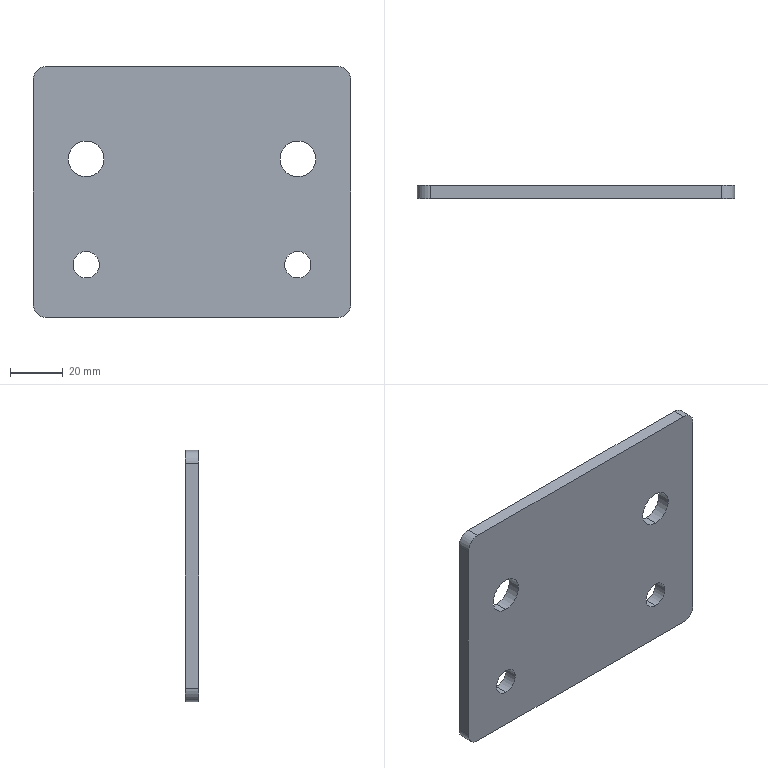Part | 1 solid | 18 faces | box 120 x 5 x 95 mm | volume 54676 mm3 | cylinder 12 | plane 6 | commonest cylinder face diameters 10 x8 13.5 x4
STEP:
#1=CARTESIAN_POINT('',(-40.,0.,-65.));
#2=VERTEX_POINT('',#1);
#3=CARTESIAN_POINT('',(-40.,0.,-75.));
#4=VERTEX_POINT('',#3);
#5=CARTESIAN_POINT('',(-40.,0.,-70.));
#6=DIRECTION('',(0.,-1.,0.));
#7=DIRECTION('',(0.,0.,-1.));
#8=AXIS2_PLACEMENT_3D('',#5,#6,#7);
#9=CIRCLE('',#8,5.);
#10=EDGE_CURVE('',#2,#4,#9,.T.);
#11=ORIENTED_EDGE('',*,*,#10,.F.);
#12=CARTESIAN_POINT('',(-40.,-5.,-65.));
#13=VERTEX_POINT('',#12);
#14=CARTESIAN_POINT('',(-40.,0.,-65.));
#15=DIRECTION('',(0.,-1.,0.));
#16=VECTOR('',#15,1000.);
#17=LINE('',#14,#16);
#18=EDGE_CURVE('',#2,#13,#17,.T.);
#19=ORIENTED_EDGE('',*,*,#18,.T.);
#20=CARTESIAN_POINT('',(-40.,-5.,-75.));
#21=VERTEX_POINT('',#20);
#22=CARTESIAN_POINT('',(-40.,-5.,-70.));
#23=DIRECTION('',(0.,-1.,0.));
#24=DIRECTION('',(0.,0.,-1.));
#25=AXIS2_PLACEMENT_3D('',#22,#23,#24);
#26=CIRCLE('',#25,5.);
#27=EDGE_CURVE('',#13,#21,#26,.T.);
#28=ORIENTED_EDGE('',*,*,#27,.T.);
#29=CARTESIAN_POINT('',(-40.,0.,-75.));
#30=DIRECTION('',(0.,-1.,0.));
#31=VECTOR('',#30,1000.);
#32=LINE('',#29,#31);
#33=EDGE_CURVE('',#4,#21,#32,.T.);
#34=ORIENTED_EDGE('',*,*,#33,.F.);
#35=EDGE_LOOP('',(#11,#19,#28,#34));
#36=FACE_OUTER_BOUND('',#35,.T.);
#37=CARTESIAN_POINT('',(-40.,0.,-70.));
#38=DIRECTION('',(0.,-1.,0.));
#39=DIRECTION('',(0.,0.,-1.));
#40=AXIS2_PLACEMENT_3D('',#37,#38,#39);
#41=CYLINDRICAL_SURFACE('',#40,5.);
#42=ADVANCED_FACE('',(#36),#41,.F.);
#43=CARTESIAN_POINT('',(40.,0.,-65.));
#44=VERTEX_POINT('',#43);
#45=CARTESIAN_POINT('',(40.,0.,-75.));
#46=VERTEX_POINT('',#45);
#47=CARTESIAN_POINT('',(40.,0.,-70.));
#48=DIRECTION('',(0.,-1.,0.));
#49=DIRECTION('',(0.,0.,-1.));
#50=AXIS2_PLACEMENT_3D('',#47,#48,#49);
#51=CIRCLE('',#50,5.);
#52=EDGE_CURVE('',#44,#46,#51,.T.);
#53=ORIENTED_EDGE('',*,*,#52,.F.);
#54=CARTESIAN_POINT('',(40.,-5.,-65.));
#55=VERTEX_POINT('',#54);
#56=CARTESIAN_POINT('',(40.,0.,-65.));
#57=DIRECTION('',(0.,-1.,0.));
#58=VECTOR('',#57,1000.);
#59=LINE('',#56,#58);
#60=EDGE_CURVE('',#44,#55,#59,.T.);
#61=ORIENTED_EDGE('',*,*,#60,.T.);
#62=CARTESIAN_POINT('',(40.,-5.,-75.));
#63=VERTEX_POINT('',#62);
#64=CARTESIAN_POINT('',(40.,-5.,-70.));
#65=DIRECTION('',(0.,-1.,0.));
#66=DIRECTION('',(0.,0.,-1.));
#67=AXIS2_PLACEMENT_3D('',#64,#65,#66);
#68=CIRCLE('',#67,5.);
#69=EDGE_CURVE('',#55,#63,#68,.T.);
#70=ORIENTED_EDGE('',*,*,#69,.T.);
#71=CARTESIAN_POINT('',(40.,0.,-75.));
#72=DIRECTION('',(0.,-1.,0.));
#73=VECTOR('',#72,1000.);
#74=LINE('',#71,#73);
#75=EDGE_CURVE('',#46,#63,#74,.T.);
#76=ORIENTED_EDGE('',*,*,#75,.F.);
#77=EDGE_LOOP('',(#53,#61,#70,#76));
#78=FACE_OUTER_BOUND('',#77,.T.);
#79=CARTESIAN_POINT('',(40.,0.,-70.));
#80=DIRECTION('',(0.,-1.,0.));
#81=DIRECTION('',(0.,0.,-1.));
#82=AXIS2_PLACEMENT_3D('',#79,#80,#81);
#83=CYLINDRICAL_SURFACE('',#82,5.);
#84=ADVANCED_FACE('',(#78),#83,.F.);
#85=CARTESIAN_POINT('',(40.,0.,-23.25));
#86=VERTEX_POINT('',#85);
#87=CARTESIAN_POINT('',(40.,0.,-36.75));
#88=VERTEX_POINT('',#87);
#89=CARTESIAN_POINT('',(40.,0.,-30.));
#90=DIRECTION('',(0.,-1.,0.));
#91=DIRECTION('',(0.,0.,-1.));
#92=AXIS2_PLACEMENT_3D('',#89,#90,#91);
#93=CIRCLE('',#92,6.75);
#94=EDGE_CURVE('',#86,#88,#93,.T.);
#95=ORIENTED_EDGE('',*,*,#94,.F.);
#96=CARTESIAN_POINT('',(40.,-5.,-23.25));
#97=VERTEX_POINT('',#96);
#98=CARTESIAN_POINT('',(40.,-5.,-23.25));
#99=DIRECTION('',(0.,-1.,0.));
#100=VECTOR('',#99,1000.);
#101=LINE('',#98,#100);
#102=EDGE_CURVE('',#86,#97,#101,.T.);
#103=ORIENTED_EDGE('',*,*,#102,.T.);
#104=CARTESIAN_POINT('',(40.,-5.,-36.75));
#105=VERTEX_POINT('',#104);
#106=CARTESIAN_POINT('',(40.,-5.,-30.));
#107=DIRECTION('',(0.,-1.,0.));
#108=DIRECTION('',(0.,0.,-1.));
#109=AXIS2_PLACEMENT_3D('',#106,#107,#108);
#110=CIRCLE('',#109,6.75);
#111=EDGE_CURVE('',#97,#105,#110,.T.);
#112=ORIENTED_EDGE('',*,*,#111,.T.);
#113=CARTESIAN_POINT('',(40.,-5.,-36.75));
#114=DIRECTION('',(0.,-1.,0.));
#115=VECTOR('',#114,1000.);
#116=LINE('',#113,#115);
#117=EDGE_CURVE('',#88,#105,#116,.T.);
#118=ORIENTED_EDGE('',*,*,#117,.F.);
#119=EDGE_LOOP('',(#95,#103,#112,#118));
#120=FACE_OUTER_BOUND('',#119,.T.);
#121=CARTESIAN_POINT('',(40.,-5.,-30.));
#122=DIRECTION('',(0.,-1.,0.));
#123=DIRECTION('',(0.,0.,-1.));
#124=AXIS2_PLACEMENT_3D('',#121,#122,#123);
#125=CYLINDRICAL_SURFACE('',#124,6.75);
#126=ADVANCED_FACE('',(#120),#125,.F.);
#127=CARTESIAN_POINT('',(-40.,0.,-23.25));
#128=VERTEX_POINT('',#127);
#129=CARTESIAN_POINT('',(-40.,0.,-36.75));
#130=VERTEX_POINT('',#129);
#131=CARTESIAN_POINT('',(-40.,0.,-30.));
#132=DIRECTION('',(0.,-1.,0.));
#133=DIRECTION('',(0.,0.,-1.));
#134=AXIS2_PLACEMENT_3D('',#131,#132,#133);
#135=CIRCLE('',#134,6.75);
#136=EDGE_CURVE('',#128,#130,#135,.T.);
#137=ORIENTED_EDGE('',*,*,#136,.F.);
#138=CARTESIAN_POINT('',(-40.,-5.,-23.25));
#139=VERTEX_POINT('',#138);
#140=CARTESIAN_POINT('',(-40.,-5.,-23.25));
#141=DIRECTION('',(0.,-1.,0.));
#142=VECTOR('',#141,1000.);
#143=LINE('',#140,#142);
#144=EDGE_CURVE('',#128,#139,#143,.T.);
#145=ORIENTED_EDGE('',*,*,#144,.T.);
#146=CARTESIAN_POINT('',(-40.,-5.,-36.75));
#147=VERTEX_POINT('',#146);
#148=CARTESIAN_POINT('',(-40.,-5.,-30.));
#149=DIRECTION('',(0.,-1.,0.));
#150=DIRECTION('',(0.,0.,-1.));
#151=AXIS2_PLACEMENT_3D('',#148,#149,#150);
#152=CIRCLE('',#151,6.75);
#153=EDGE_CURVE('',#139,#147,#152,.T.);
#154=ORIENTED_EDGE('',*,*,#153,.T.);
#155=CARTESIAN_POINT('',(-40.,-5.,-36.75));
#156=DIRECTION('',(0.,-1.,0.));
#157=VECTOR('',#156,1000.);
#158=LINE('',#155,#157);
#159=EDGE_CURVE('',#130,#147,#158,.T.);
#160=ORIENTED_EDGE('',*,*,#159,.F.);
#161=EDGE_LOOP('',(#137,#145,#154,#160));
#162=FACE_OUTER_BOUND('',#161,.T.);
#163=CARTESIAN_POINT('',(-40.,-5.,-30.));
#164=DIRECTION('',(0.,-1.,0.));
#165=DIRECTION('',(0.,0.,-1.));
#166=AXIS2_PLACEMENT_3D('',#163,#164,#165);
#167=CYLINDRICAL_SURFACE('',#166,6.75);
#168=ADVANCED_FACE('',(#162),#167,.F.);
#169=CARTESIAN_POINT('',(60.,0.,0.));
#170=VERTEX_POINT('',#169);
#171=CARTESIAN_POINT('',(60.,0.,-85.));
#172=VERTEX_POINT('',#171);
#173=CARTESIAN_POINT('',(60.,0.,50.));
#174=DIRECTION('',(0.,0.,-1.));
#175=VECTOR('',#174,1000.);
#176=LINE('',#173,#175);
#177=EDGE_CURVE('',#170,#172,#176,.T.);
#178=ORIENTED_EDGE('',*,*,#177,.F.);
#179=CARTESIAN_POINT('',(60.,-5.,0.));
#180=VERTEX_POINT('',#179);
#181=CARTESIAN_POINT('',(60.,-5.,0.));
#182=DIRECTION('',(0.,-1.,0.));
#183=VECTOR('',#182,1000.);
#184=LINE('',#181,#183);
#185=EDGE_CURVE('',#170,#180,#184,.T.);
#186=ORIENTED_EDGE('',*,*,#185,.T.);
#187=CARTESIAN_POINT('',(60.,-5.,-85.));
#188=VERTEX_POINT('',#187);
#189=CARTESIAN_POINT('',(60.,-5.,50.));
#190=DIRECTION('',(0.,0.,-1.));
#191=VECTOR('',#190,1000.);
#192=LINE('',#189,#191);
#193=EDGE_CURVE('',#180,#188,#192,.T.);
#194=ORIENTED_EDGE('',*,*,#193,.T.);
#195=CARTESIAN_POINT('',(60.,-5.,-85.));
#196=DIRECTION('',(0.,1.,0.));
#197=VECTOR('',#196,1000.);
#198=LINE('',#195,#197);
#199=EDGE_CURVE('',#188,#172,#198,.T.);
#200=ORIENTED_EDGE('',*,*,#199,.T.);
#201=EDGE_LOOP('',(#178,#186,#194,#200));
#202=FACE_OUTER_BOUND('',#201,.T.);
#203=CARTESIAN_POINT('',(60.,-5.,50.));
#204=DIRECTION('',(1.,0.,0.));
#205=DIRECTION('',(0.,0.,-1.));
#206=AXIS2_PLACEMENT_3D('',#203,#204,#205);
#207=PLANE('',#206);
#208=ADVANCED_FACE('',(#202),#207,.T.);
#209=CARTESIAN_POINT('',(-60.,0.,-85.));
#210=VERTEX_POINT('',#209);
#211=CARTESIAN_POINT('',(-60.,0.,0.));
#212=VERTEX_POINT('',#211);
#213=CARTESIAN_POINT('',(-60.,0.,50.));
#214=DIRECTION('',(0.,0.,1.));
#215=VECTOR('',#214,1000.);
#216=LINE('',#213,#215);
#217=EDGE_CURVE('',#210,#212,#216,.T.);
#218=ORIENTED_EDGE('',*,*,#217,.F.);
#219=CARTESIAN_POINT('',(-60.,-5.,-85.));
#220=VERTEX_POINT('',#219);
#221=CARTESIAN_POINT('',(-60.,-5.,-85.));
#222=DIRECTION('',(0.,-1.,0.));
#223=VECTOR('',#222,1000.);
#224=LINE('',#221,#223);
#225=EDGE_CURVE('',#210,#220,#224,.T.);
#226=ORIENTED_EDGE('',*,*,#225,.T.);
#227=CARTESIAN_POINT('',(-60.,-5.,0.));
#228=VERTEX_POINT('',#227);
#229=CARTESIAN_POINT('',(-60.,-5.,50.));
#230=DIRECTION('',(0.,0.,1.));
#231=VECTOR('',#230,1000.);
#232=LINE('',#229,#231);
#233=EDGE_CURVE('',#220,#228,#232,.T.);
#234=ORIENTED_EDGE('',*,*,#233,.T.);
#235=CARTESIAN_POINT('',(-60.,0.,0.));
#236=DIRECTION('',(0.,1.,0.));
#237=VECTOR('',#236,1000.);
#238=LINE('',#235,#237);
#239=EDGE_CURVE('',#228,#212,#238,.T.);
#240=ORIENTED_EDGE('',*,*,#239,.T.);
#241=EDGE_LOOP('',(#218,#226,#234,#240));
#242=FACE_OUTER_BOUND('',#241,.T.);
#243=CARTESIAN_POINT('',(-60.,-5.,50.));
#244=DIRECTION('',(-1.,0.,0.));
#245=DIRECTION('',(0.,0.,1.));
#246=AXIS2_PLACEMENT_3D('',#243,#244,#245);
#247=PLANE('',#246);
#248=ADVANCED_FACE('',(#242),#247,.T.);
#249=CARTESIAN_POINT('',(55.,-5.,-90.));
#250=VERTEX_POINT('',#249);
#251=CARTESIAN_POINT('',(-55.,-5.,-90.));
#252=VERTEX_POINT('',#251);
#253=CARTESIAN_POINT('',(-60.,-5.,-90.));
#254=DIRECTION('',(-1.,0.,0.));
#255=VECTOR('',#254,1000.);
#256=LINE('',#253,#255);
#257=EDGE_CURVE('',#250,#252,#256,.T.);
#258=ORIENTED_EDGE('',*,*,#257,.T.);
#259=CARTESIAN_POINT('',(-55.,0.,-90.));
#260=VERTEX_POINT('',#259);
#261=CARTESIAN_POINT('',(-55.,-5.,-90.));
#262=DIRECTION('',(0.,1.,0.));
#263=VECTOR('',#262,1000.);
#264=LINE('',#261,#263);
#265=EDGE_CURVE('',#252,#260,#264,.T.);
#266=ORIENTED_EDGE('',*,*,#265,.T.);
#267=CARTESIAN_POINT('',(55.,0.,-90.));
#268=VERTEX_POINT('',#267);
#269=CARTESIAN_POINT('',(-60.,0.,-90.));
#270=DIRECTION('',(-1.,0.,0.));
#271=VECTOR('',#270,1000.);
#272=LINE('',#269,#271);
#273=EDGE_CURVE('',#268,#260,#272,.T.);
#274=ORIENTED_EDGE('',*,*,#273,.F.);
#275=CARTESIAN_POINT('',(55.,-5.,-90.));
#276=DIRECTION('',(0.,-1.,0.));
#277=VECTOR('',#276,1000.);
#278=LINE('',#275,#277);
#279=EDGE_CURVE('',#268,#250,#278,.T.);
#280=ORIENTED_EDGE('',*,*,#279,.T.);
#281=EDGE_LOOP('',(#258,#266,#274,#280));
#282=FACE_OUTER_BOUND('',#281,.T.);
#283=CARTESIAN_POINT('',(-60.,-5.,-90.));
#284=DIRECTION('',(0.,0.,-1.));
#285=DIRECTION('',(-1.,0.,0.));
#286=AXIS2_PLACEMENT_3D('',#283,#284,#285);
#287=PLANE('',#286);
#288=ADVANCED_FACE('',(#282),#287,.T.);
#289=CARTESIAN_POINT('',(-40.,-5.,-70.));
#290=DIRECTION('',(0.,-1.,0.));
#291=DIRECTION('',(0.,0.,-1.));
#292=AXIS2_PLACEMENT_3D('',#289,#290,#291);
#293=CIRCLE('',#292,5.);
#294=EDGE_CURVE('',#21,#13,#293,.T.);
#295=ORIENTED_EDGE('',*,*,#294,.F.);
#296=ORIENTED_EDGE('',*,*,#27,.F.);
#297=EDGE_LOOP('',(#295,#296));
#298=FACE_BOUND('',#297,.T.);
#299=CARTESIAN_POINT('',(40.,-5.,-70.));
#300=DIRECTION('',(0.,-1.,0.));
#301=DIRECTION('',(0.,0.,-1.));
#302=AXIS2_PLACEMENT_3D('',#299,#300,#301);
#303=CIRCLE('',#302,5.);
#304=EDGE_CURVE('',#63,#55,#303,.T.);
#305=ORIENTED_EDGE('',*,*,#304,.F.);
#306=ORIENTED_EDGE('',*,*,#69,.F.);
#307=EDGE_LOOP('',(#305,#306));
#308=FACE_BOUND('',#307,.T.);
#309=ORIENTED_EDGE('',*,*,#233,.F.);
#310=CARTESIAN_POINT('',(-55.,-5.,-85.));
#311=DIRECTION('',(0.,-1.,0.));
#312=DIRECTION('',(0.,0.,-1.));
#313=AXIS2_PLACEMENT_3D('',#310,#311,#312);
#314=CIRCLE('',#313,5.);
#315=EDGE_CURVE('',#220,#252,#314,.T.);
#316=ORIENTED_EDGE('',*,*,#315,.T.);
#317=ORIENTED_EDGE('',*,*,#257,.F.);
#318=CARTESIAN_POINT('',(55.,-5.,-85.));
#319=DIRECTION('',(0.,-1.,0.));
#320=DIRECTION('',(0.,0.,-1.));
#321=AXIS2_PLACEMENT_3D('',#318,#319,#320);
#322=CIRCLE('',#321,5.);
#323=EDGE_CURVE('',#250,#188,#322,.T.);
#324=ORIENTED_EDGE('',*,*,#323,.T.);
#325=ORIENTED_EDGE('',*,*,#193,.F.);
#326=CARTESIAN_POINT('',(55.,-5.,5.));
#327=VERTEX_POINT('',#326);
#328=CARTESIAN_POINT('',(55.,-5.,0.));
#329=DIRECTION('',(0.,-1.,0.));
#330=DIRECTION('',(0.,0.,-1.));
#331=AXIS2_PLACEMENT_3D('',#328,#329,#330);
#332=CIRCLE('',#331,5.);
#333=EDGE_CURVE('',#180,#327,#332,.T.);
#334=ORIENTED_EDGE('',*,*,#333,.T.);
#335=CARTESIAN_POINT('',(-55.,-5.,5.));
#336=VERTEX_POINT('',#335);
#337=CARTESIAN_POINT('',(-60.,-5.,5.));
#338=DIRECTION('',(1.,0.,0.));
#339=VECTOR('',#338,1000.);
#340=LINE('',#337,#339);
#341=EDGE_CURVE('',#336,#327,#340,.T.);
#342=ORIENTED_EDGE('',*,*,#341,.F.);
#343=CARTESIAN_POINT('',(-55.,-5.,0.));
#344=DIRECTION('',(0.,-1.,0.));
#345=DIRECTION('',(0.,0.,-1.));
#346=AXIS2_PLACEMENT_3D('',#343,#344,#345);
#347=CIRCLE('',#346,5.);
#348=EDGE_CURVE('',#336,#228,#347,.T.);
#349=ORIENTED_EDGE('',*,*,#348,.T.);
#350=EDGE_LOOP('',(#309,#316,#317,#324,#325,#334,#342,#349));
#351=FACE_OUTER_BOUND('',#350,.T.);
#352=CARTESIAN_POINT('',(40.,-5.,-30.));
#353=DIRECTION('',(0.,-1.,0.));
#354=DIRECTION('',(0.,0.,-1.));
#355=AXIS2_PLACEMENT_3D('',#352,#353,#354);
#356=CIRCLE('',#355,6.75);
#357=EDGE_CURVE('',#105,#97,#356,.T.);
#358=ORIENTED_EDGE('',*,*,#357,.F.);
#359=ORIENTED_EDGE('',*,*,#111,.F.);
#360=EDGE_LOOP('',(#358,#359));
#361=FACE_BOUND('',#360,.T.);
#362=CARTESIAN_POINT('',(-40.,-5.,-30.));
#363=DIRECTION('',(0.,-1.,0.));
#364=DIRECTION('',(0.,0.,-1.));
#365=AXIS2_PLACEMENT_3D('',#362,#363,#364);
#366=CIRCLE('',#365,6.75);
#367=EDGE_CURVE('',#147,#139,#366,.T.);
#368=ORIENTED_EDGE('',*,*,#367,.F.);
#369=ORIENTED_EDGE('',*,*,#153,.F.);
#370=EDGE_LOOP('',(#368,#369));
#371=FACE_BOUND('',#370,.T.);
#372=CARTESIAN_POINT('',(0.,-5.,0.));
#373=DIRECTION('',(0.,-1.,0.));
#374=DIRECTION('',(0.,0.,-1.));
#375=AXIS2_PLACEMENT_3D('',#372,#373,#374);
#376=PLANE('',#375);
#377=ADVANCED_FACE('',(#298,#308,#351,#361,#371),#376,.T.);
#378=CARTESIAN_POINT('',(-40.,0.,-70.));
#379=DIRECTION('',(0.,-1.,0.));
#380=DIRECTION('',(0.,0.,-1.));
#381=AXIS2_PLACEMENT_3D('',#378,#379,#380);
#382=CIRCLE('',#381,5.);
#383=EDGE_CURVE('',#4,#2,#382,.T.);
#384=ORIENTED_EDGE('',*,*,#383,.T.);
#385=ORIENTED_EDGE('',*,*,#10,.T.);
#386=EDGE_LOOP('',(#384,#385));
#387=FACE_BOUND('',#386,.T.);
#388=CARTESIAN_POINT('',(40.,0.,-70.));
#389=DIRECTION('',(0.,-1.,0.));
#390=DIRECTION('',(0.,0.,-1.));
#391=AXIS2_PLACEMENT_3D('',#388,#389,#390);
#392=CIRCLE('',#391,5.);
#393=EDGE_CURVE('',#46,#44,#392,.T.);
#394=ORIENTED_EDGE('',*,*,#393,.T.);
#395=ORIENTED_EDGE('',*,*,#52,.T.);
#396=EDGE_LOOP('',(#394,#395));
#397=FACE_BOUND('',#396,.T.);
#398=CARTESIAN_POINT('',(40.,0.,-30.));
#399=DIRECTION('',(0.,-1.,0.));
#400=DIRECTION('',(0.,0.,-1.));
#401=AXIS2_PLACEMENT_3D('',#398,#399,#400);
#402=CIRCLE('',#401,6.75);
#403=EDGE_CURVE('',#88,#86,#402,.T.);
#404=ORIENTED_EDGE('',*,*,#403,.T.);
#405=ORIENTED_EDGE('',*,*,#94,.T.);
#406=EDGE_LOOP('',(#404,#405));
#407=FACE_BOUND('',#406,.T.);
#408=CARTESIAN_POINT('',(-40.,0.,-30.));
#409=DIRECTION('',(0.,-1.,0.));
#410=DIRECTION('',(0.,0.,-1.));
#411=AXIS2_PLACEMENT_3D('',#408,#409,#410);
#412=CIRCLE('',#411,6.75);
#413=EDGE_CURVE('',#130,#128,#412,.T.);
#414=ORIENTED_EDGE('',*,*,#413,.T.);
#415=ORIENTED_EDGE('',*,*,#136,.T.);
#416=EDGE_LOOP('',(#414,#415));
#417=FACE_BOUND('',#416,.T.);
#418=ORIENTED_EDGE('',*,*,#273,.T.);
#419=CARTESIAN_POINT('',(-55.,0.,-85.));
#420=DIRECTION('',(0.,1.,0.));
#421=DIRECTION('',(0.,0.,-1.));
#422=AXIS2_PLACEMENT_3D('',#419,#420,#421);
#423=CIRCLE('',#422,5.);
#424=EDGE_CURVE('',#260,#210,#423,.T.);
#425=ORIENTED_EDGE('',*,*,#424,.T.);
#426=ORIENTED_EDGE('',*,*,#217,.T.);
#427=CARTESIAN_POINT('',(-55.,0.,5.));
#428=VERTEX_POINT('',#427);
#429=CARTESIAN_POINT('',(-55.,0.,0.));
#430=DIRECTION('',(0.,1.,0.));
#431=DIRECTION('',(0.,0.,-1.));
#432=AXIS2_PLACEMENT_3D('',#429,#430,#431);
#433=CIRCLE('',#432,5.);
#434=EDGE_CURVE('',#212,#428,#433,.T.);
#435=ORIENTED_EDGE('',*,*,#434,.T.);
#436=CARTESIAN_POINT('',(55.,0.,5.));
#437=VERTEX_POINT('',#436);
#438=CARTESIAN_POINT('',(-60.,0.,5.));
#439=DIRECTION('',(1.,0.,0.));
#440=VECTOR('',#439,1000.);
#441=LINE('',#438,#440);
#442=EDGE_CURVE('',#428,#437,#441,.T.);
#443=ORIENTED_EDGE('',*,*,#442,.T.);
#444=CARTESIAN_POINT('',(55.,0.,0.));
#445=DIRECTION('',(0.,1.,0.));
#446=DIRECTION('',(0.,0.,-1.));
#447=AXIS2_PLACEMENT_3D('',#444,#445,#446);
#448=CIRCLE('',#447,5.);
#449=EDGE_CURVE('',#437,#170,#448,.T.);
#450=ORIENTED_EDGE('',*,*,#449,.T.);
#451=ORIENTED_EDGE('',*,*,#177,.T.);
#452=CARTESIAN_POINT('',(55.,0.,-85.));
#453=DIRECTION('',(0.,1.,0.));
#454=DIRECTION('',(0.,0.,-1.));
#455=AXIS2_PLACEMENT_3D('',#452,#453,#454);
#456=CIRCLE('',#455,5.);
#457=EDGE_CURVE('',#172,#268,#456,.T.);
#458=ORIENTED_EDGE('',*,*,#457,.T.);
#459=EDGE_LOOP('',(#418,#425,#426,#435,#443,#450,#451,#458));
#460=FACE_OUTER_BOUND('',#459,.T.);
#461=CARTESIAN_POINT('',(0.,0.,0.));
#462=DIRECTION('',(0.,-1.,0.));
#463=DIRECTION('',(0.,0.,-1.));
#464=AXIS2_PLACEMENT_3D('',#461,#462,#463);
#465=PLANE('',#464);
#466=ADVANCED_FACE('',(#387,#397,#407,#417,#460),#465,.F.);
#467=ORIENTED_EDGE('',*,*,#144,.F.);
#468=ORIENTED_EDGE('',*,*,#413,.F.);
#469=ORIENTED_EDGE('',*,*,#159,.T.);
#470=ORIENTED_EDGE('',*,*,#367,.T.);
#471=EDGE_LOOP('',(#467,#468,#469,#470));
#472=FACE_OUTER_BOUND('',#471,.T.);
#473=CARTESIAN_POINT('',(-40.,-5.,-30.));
#474=DIRECTION('',(0.,-1.,0.));
#475=DIRECTION('',(0.,0.,-1.));
#476=AXIS2_PLACEMENT_3D('',#473,#474,#475);
#477=CYLINDRICAL_SURFACE('',#476,6.75);
#478=ADVANCED_FACE('',(#472),#477,.F.);
#479=ORIENTED_EDGE('',*,*,#102,.F.);
#480=ORIENTED_EDGE('',*,*,#403,.F.);
#481=ORIENTED_EDGE('',*,*,#117,.T.);
#482=ORIENTED_EDGE('',*,*,#357,.T.);
#483=EDGE_LOOP('',(#479,#480,#481,#482));
#484=FACE_OUTER_BOUND('',#483,.T.);
#485=CARTESIAN_POINT('',(40.,-5.,-30.));
#486=DIRECTION('',(0.,-1.,0.));
#487=DIRECTION('',(0.,0.,-1.));
#488=AXIS2_PLACEMENT_3D('',#485,#486,#487);
#489=CYLINDRICAL_SURFACE('',#488,6.75);
#490=ADVANCED_FACE('',(#484),#489,.F.);
#491=ORIENTED_EDGE('',*,*,#442,.F.);
#492=CARTESIAN_POINT('',(-55.,-5.,5.));
#493=DIRECTION('',(0.,-1.,0.));
#494=VECTOR('',#493,1000.);
#495=LINE('',#492,#494);
#496=EDGE_CURVE('',#428,#336,#495,.T.);
#497=ORIENTED_EDGE('',*,*,#496,.T.);
#498=ORIENTED_EDGE('',*,*,#341,.T.);
#499=CARTESIAN_POINT('',(55.,0.,5.));
#500=DIRECTION('',(0.,1.,0.));
#501=VECTOR('',#500,1000.);
#502=LINE('',#499,#501);
#503=EDGE_CURVE('',#327,#437,#502,.T.);
#504=ORIENTED_EDGE('',*,*,#503,.T.);
#505=EDGE_LOOP('',(#491,#497,#498,#504));
#506=FACE_OUTER_BOUND('',#505,.T.);
#507=CARTESIAN_POINT('',(-60.,0.,5.));
#508=DIRECTION('',(0.,0.,-1.));
#509=DIRECTION('',(-1.,0.,0.));
#510=AXIS2_PLACEMENT_3D('',#507,#508,#509);
#511=PLANE('',#510);
#512=ADVANCED_FACE('',(#506),#511,.F.);
#513=ORIENTED_EDGE('',*,*,#315,.F.);
#514=ORIENTED_EDGE('',*,*,#225,.F.);
#515=ORIENTED_EDGE('',*,*,#424,.F.);
#516=ORIENTED_EDGE('',*,*,#265,.F.);
#517=EDGE_LOOP('',(#513,#514,#515,#516));
#518=FACE_OUTER_BOUND('',#517,.T.);
#519=CARTESIAN_POINT('',(-55.,-5.,-85.));
#520=DIRECTION('',(0.,1.,0.));
#521=DIRECTION('',(0.,0.,1.));
#522=AXIS2_PLACEMENT_3D('',#519,#520,#521);
#523=CYLINDRICAL_SURFACE('',#522,5.);
#524=ADVANCED_FACE('',(#518),#523,.T.);
#525=ORIENTED_EDGE('',*,*,#434,.F.);
#526=ORIENTED_EDGE('',*,*,#239,.F.);
#527=ORIENTED_EDGE('',*,*,#348,.F.);
#528=ORIENTED_EDGE('',*,*,#496,.F.);
#529=EDGE_LOOP('',(#525,#526,#527,#528));
#530=FACE_OUTER_BOUND('',#529,.T.);
#531=CARTESIAN_POINT('',(-55.,0.,0.));
#532=DIRECTION('',(0.,1.,0.));
#533=DIRECTION('',(0.,0.,1.));
#534=AXIS2_PLACEMENT_3D('',#531,#532,#533);
#535=CYLINDRICAL_SURFACE('',#534,5.);
#536=ADVANCED_FACE('',(#530),#535,.T.);
#537=ORIENTED_EDGE('',*,*,#449,.F.);
#538=ORIENTED_EDGE('',*,*,#503,.F.);
#539=ORIENTED_EDGE('',*,*,#333,.F.);
#540=ORIENTED_EDGE('',*,*,#185,.F.);
#541=EDGE_LOOP('',(#537,#538,#539,#540));
#542=FACE_OUTER_BOUND('',#541,.T.);
#543=CARTESIAN_POINT('',(55.,-5.,0.));
#544=DIRECTION('',(0.,1.,0.));
#545=DIRECTION('',(0.,0.,1.));
#546=AXIS2_PLACEMENT_3D('',#543,#544,#545);
#547=CYLINDRICAL_SURFACE('',#546,5.);
#548=ADVANCED_FACE('',(#542),#547,.T.);
#549=ORIENTED_EDGE('',*,*,#323,.F.);
#550=ORIENTED_EDGE('',*,*,#279,.F.);
#551=ORIENTED_EDGE('',*,*,#457,.F.);
#552=ORIENTED_EDGE('',*,*,#199,.F.);
#553=EDGE_LOOP('',(#549,#550,#551,#552));
#554=FACE_OUTER_BOUND('',#553,.T.);
#555=CARTESIAN_POINT('',(55.,-5.,-85.));
#556=DIRECTION('',(0.,1.,0.));
#557=DIRECTION('',(0.,0.,1.));
#558=AXIS2_PLACEMENT_3D('',#555,#556,#557);
#559=CYLINDRICAL_SURFACE('',#558,5.);
#560=ADVANCED_FACE('',(#554),#559,.T.);
#561=ORIENTED_EDGE('',*,*,#60,.F.);
#562=ORIENTED_EDGE('',*,*,#393,.F.);
#563=ORIENTED_EDGE('',*,*,#75,.T.);
#564=ORIENTED_EDGE('',*,*,#304,.T.);
#565=EDGE_LOOP('',(#561,#562,#563,#564));
#566=FACE_OUTER_BOUND('',#565,.T.);
#567=CARTESIAN_POINT('',(40.,0.,-70.));
#568=DIRECTION('',(0.,-1.,0.));
#569=DIRECTION('',(0.,0.,-1.));
#570=AXIS2_PLACEMENT_3D('',#567,#568,#569);
#571=CYLINDRICAL_SURFACE('',#570,5.);
#572=ADVANCED_FACE('',(#566),#571,.F.);
#573=ORIENTED_EDGE('',*,*,#18,.F.);
#574=ORIENTED_EDGE('',*,*,#383,.F.);
#575=ORIENTED_EDGE('',*,*,#33,.T.);
#576=ORIENTED_EDGE('',*,*,#294,.T.);
#577=EDGE_LOOP('',(#573,#574,#575,#576));
#578=FACE_OUTER_BOUND('',#577,.T.);
#579=CARTESIAN_POINT('',(-40.,0.,-70.));
#580=DIRECTION('',(0.,-1.,0.));
#581=DIRECTION('',(0.,0.,-1.));
#582=AXIS2_PLACEMENT_3D('',#579,#580,#581);
#583=CYLINDRICAL_SURFACE('',#582,5.);
#584=ADVANCED_FACE('',(#578),#583,.F.);
#585=CLOSED_SHELL('',(#42,#84,#126,#168,#208,#248,#288,#377,#466,#478,#490,#512,#524,#536,#548,#560,#572,#584));
#586=MANIFOLD_SOLID_BREP('',#585);
#587=CARTESIAN_POINT('',(0.,0.,0.));
#588=DIRECTION('',(0.,0.,1.));
#589=DIRECTION('',(1.,0.,0.));
#590=AXIS2_PLACEMENT_3D('',#587,#588,#589);
#591=(LENGTH_UNIT()NAMED_UNIT(*)SI_UNIT(.MILLI.,.METRE.));
#592=UNCERTAINTY_MEASURE_WITH_UNIT(LENGTH_MEASURE(0.00001),#591,'','');
#593=(NAMED_UNIT(*)PLANE_ANGLE_UNIT()SI_UNIT($,.RADIAN.));
#594=(NAMED_UNIT(*)SI_UNIT($,.STERADIAN.)SOLID_ANGLE_UNIT());
#595=(GEOMETRIC_REPRESENTATION_CONTEXT(3)GLOBAL_UNCERTAINTY_ASSIGNED_CONTEXT((#592))GLOBAL_UNIT_ASSIGNED_CONTEXT((#591,#593,#594))REPRESENTATION_CONTEXT('',''));
#596=ADVANCED_BREP_SHAPE_REPRESENTATION('',(#586,#590),#595);